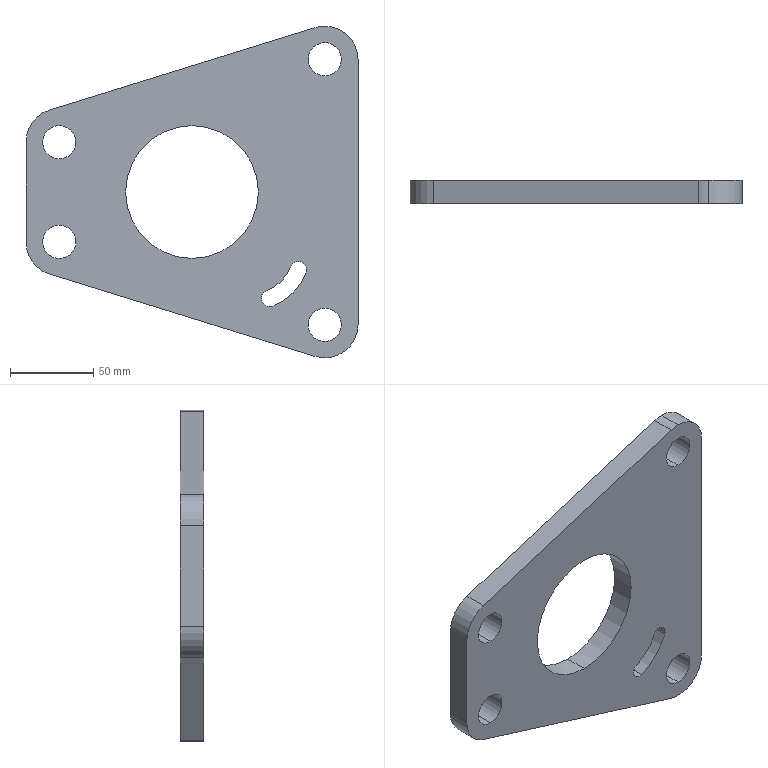Part | SolidWorks | features FlatPattern 1, SMBaseFlange 1, SheetMetal 1 | 1 solid | 26 faces | box 200 x 14 x 199.722 mm | volume 327210 mm3 | cylinder 20 | plane 6 | commonest cylinder face diameters 20 x8 40 x5 10 x3 80 x2 49 x1 69 x1
STEP:
#1=CARTESIAN_POINT('',(180.,-14.,70.));
#2=VERTEX_POINT('',#1);
#3=CARTESIAN_POINT('',(180.,-14.,90.));
#4=VERTEX_POINT('',#3);
#5=CARTESIAN_POINT('',(180.,-14.,80.));
#6=DIRECTION('',(0.,1.,0.));
#7=DIRECTION('',(0.,0.,-1.));
#8=AXIS2_PLACEMENT_3D('',#5,#6,#7);
#9=CIRCLE('',#8,10.);
#10=EDGE_CURVE('',#2,#4,#9,.T.);
#11=ORIENTED_EDGE('',*,*,#10,.F.);
#12=CARTESIAN_POINT('',(180.,0.,70.));
#13=VERTEX_POINT('',#12);
#14=CARTESIAN_POINT('',(180.,-14.,70.));
#15=DIRECTION('',(0.,1.,0.));
#16=VECTOR('',#15,1000.);
#17=LINE('',#14,#16);
#18=EDGE_CURVE('',#2,#13,#17,.T.);
#19=ORIENTED_EDGE('',*,*,#18,.T.);
#20=CARTESIAN_POINT('',(180.,0.,90.));
#21=VERTEX_POINT('',#20);
#22=CARTESIAN_POINT('',(180.,0.,80.));
#23=DIRECTION('',(0.,1.,0.));
#24=DIRECTION('',(0.,0.,-1.));
#25=AXIS2_PLACEMENT_3D('',#22,#23,#24);
#26=CIRCLE('',#25,10.);
#27=EDGE_CURVE('',#13,#21,#26,.T.);
#28=ORIENTED_EDGE('',*,*,#27,.T.);
#29=CARTESIAN_POINT('',(180.,-14.,90.));
#30=DIRECTION('',(0.,1.,0.));
#31=VECTOR('',#30,1000.);
#32=LINE('',#29,#31);
#33=EDGE_CURVE('',#4,#21,#32,.T.);
#34=ORIENTED_EDGE('',*,*,#33,.F.);
#35=EDGE_LOOP('',(#11,#19,#28,#34));
#36=FACE_OUTER_BOUND('',#35,.T.);
#37=CARTESIAN_POINT('',(180.,-14.,80.));
#38=DIRECTION('',(0.,1.,0.));
#39=DIRECTION('',(0.,0.,1.));
#40=AXIS2_PLACEMENT_3D('',#37,#38,#39);
#41=CYLINDRICAL_SURFACE('',#40,10.);
#42=ADVANCED_FACE('',(#36),#41,.F.);
#43=CARTESIAN_POINT('',(164.,-14.,-42.));
#44=VERTEX_POINT('',#43);
#45=CARTESIAN_POINT('',(168.669,-14.,-48.788));
#46=VERTEX_POINT('',#45);
#47=CARTESIAN_POINT('',(164.,-14.,-47.));
#48=DIRECTION('',(0.,1.,0.));
#49=DIRECTION('',(0.,0.,1.));
#50=AXIS2_PLACEMENT_3D('',#47,#48,#49);
#51=CIRCLE('',#50,5.);
#52=EDGE_CURVE('',#44,#46,#51,.T.);
#53=ORIENTED_EDGE('',*,*,#52,.F.);
#54=CARTESIAN_POINT('',(164.,0.,-42.));
#55=VERTEX_POINT('',#54);
#56=CARTESIAN_POINT('',(164.,-14.,-42.));
#57=DIRECTION('',(0.,1.,0.));
#58=VECTOR('',#57,1000.);
#59=LINE('',#56,#58);
#60=EDGE_CURVE('',#44,#55,#59,.T.);
#61=ORIENTED_EDGE('',*,*,#60,.T.);
#62=CARTESIAN_POINT('',(168.669,0.,-48.788));
#63=VERTEX_POINT('',#62);
#64=CARTESIAN_POINT('',(164.,0.,-47.));
#65=DIRECTION('',(0.,1.,0.));
#66=DIRECTION('',(0.,0.,1.));
#67=AXIS2_PLACEMENT_3D('',#64,#65,#66);
#68=CIRCLE('',#67,5.);
#69=EDGE_CURVE('',#55,#63,#68,.T.);
#70=ORIENTED_EDGE('',*,*,#69,.T.);
#71=CARTESIAN_POINT('',(168.669,-14.,-48.788));
#72=DIRECTION('',(0.,1.,0.));
#73=VECTOR('',#72,1000.);
#74=LINE('',#71,#73);
#75=EDGE_CURVE('',#46,#63,#74,.T.);
#76=ORIENTED_EDGE('',*,*,#75,.F.);
#77=EDGE_LOOP('',(#53,#61,#70,#76));
#78=FACE_OUTER_BOUND('',#77,.T.);
#79=CARTESIAN_POINT('',(164.,-14.,-47.));
#80=DIRECTION('',(0.,1.,0.));
#81=DIRECTION('',(0.,0.,1.));
#82=AXIS2_PLACEMENT_3D('',#79,#80,#81);
#83=CYLINDRICAL_SURFACE('',#82,5.);
#84=ADVANCED_FACE('',(#78),#83,.F.);
#85=CARTESIAN_POINT('',(20.,-14.,20.));
#86=VERTEX_POINT('',#85);
#87=CARTESIAN_POINT('',(20.,-14.,40.));
#88=VERTEX_POINT('',#87);
#89=CARTESIAN_POINT('',(20.,-14.,30.));
#90=DIRECTION('',(0.,1.,0.));
#91=DIRECTION('',(0.,0.,-1.));
#92=AXIS2_PLACEMENT_3D('',#89,#90,#91);
#93=CIRCLE('',#92,10.);
#94=EDGE_CURVE('',#86,#88,#93,.T.);
#95=ORIENTED_EDGE('',*,*,#94,.F.);
#96=CARTESIAN_POINT('',(20.,0.,20.));
#97=VERTEX_POINT('',#96);
#98=CARTESIAN_POINT('',(20.,-14.,20.));
#99=DIRECTION('',(0.,1.,0.));
#100=VECTOR('',#99,1000.);
#101=LINE('',#98,#100);
#102=EDGE_CURVE('',#86,#97,#101,.T.);
#103=ORIENTED_EDGE('',*,*,#102,.T.);
#104=CARTESIAN_POINT('',(20.,0.,40.));
#105=VERTEX_POINT('',#104);
#106=CARTESIAN_POINT('',(20.,0.,30.));
#107=DIRECTION('',(0.,1.,0.));
#108=DIRECTION('',(0.,0.,-1.));
#109=AXIS2_PLACEMENT_3D('',#106,#107,#108);
#110=CIRCLE('',#109,10.);
#111=EDGE_CURVE('',#97,#105,#110,.T.);
#112=ORIENTED_EDGE('',*,*,#111,.T.);
#113=CARTESIAN_POINT('',(20.,-14.,40.));
#114=DIRECTION('',(0.,1.,0.));
#115=VECTOR('',#114,1000.);
#116=LINE('',#113,#115);
#117=EDGE_CURVE('',#88,#105,#116,.T.);
#118=ORIENTED_EDGE('',*,*,#117,.F.);
#119=EDGE_LOOP('',(#95,#103,#112,#118));
#120=FACE_OUTER_BOUND('',#119,.T.);
#121=CARTESIAN_POINT('',(20.,-14.,30.));
#122=DIRECTION('',(0.,1.,0.));
#123=DIRECTION('',(0.,0.,1.));
#124=AXIS2_PLACEMENT_3D('',#121,#122,#123);
#125=CYLINDRICAL_SURFACE('',#124,10.);
#126=ADVANCED_FACE('',(#120),#125,.F.);
#127=CARTESIAN_POINT('',(180.,-14.,-90.));
#128=VERTEX_POINT('',#127);
#129=CARTESIAN_POINT('',(180.,-14.,-70.));
#130=VERTEX_POINT('',#129);
#131=CARTESIAN_POINT('',(180.,-14.,-80.));
#132=DIRECTION('',(0.,1.,0.));
#133=DIRECTION('',(0.,0.,1.));
#134=AXIS2_PLACEMENT_3D('',#131,#132,#133);
#135=CIRCLE('',#134,10.);
#136=EDGE_CURVE('',#128,#130,#135,.T.);
#137=ORIENTED_EDGE('',*,*,#136,.F.);
#138=CARTESIAN_POINT('',(180.,0.,-90.));
#139=VERTEX_POINT('',#138);
#140=CARTESIAN_POINT('',(180.,-14.,-90.));
#141=DIRECTION('',(0.,1.,0.));
#142=VECTOR('',#141,1000.);
#143=LINE('',#140,#142);
#144=EDGE_CURVE('',#128,#139,#143,.T.);
#145=ORIENTED_EDGE('',*,*,#144,.T.);
#146=CARTESIAN_POINT('',(180.,0.,-70.));
#147=VERTEX_POINT('',#146);
#148=CARTESIAN_POINT('',(180.,0.,-80.));
#149=DIRECTION('',(0.,1.,0.));
#150=DIRECTION('',(0.,0.,1.));
#151=AXIS2_PLACEMENT_3D('',#148,#149,#150);
#152=CIRCLE('',#151,10.);
#153=EDGE_CURVE('',#139,#147,#152,.T.);
#154=ORIENTED_EDGE('',*,*,#153,.T.);
#155=CARTESIAN_POINT('',(180.,-14.,-70.));
#156=DIRECTION('',(0.,1.,0.));
#157=VECTOR('',#156,1000.);
#158=LINE('',#155,#157);
#159=EDGE_CURVE('',#130,#147,#158,.T.);
#160=ORIENTED_EDGE('',*,*,#159,.F.);
#161=EDGE_LOOP('',(#137,#145,#154,#160));
#162=FACE_OUTER_BOUND('',#161,.T.);
#163=CARTESIAN_POINT('',(180.,-14.,-80.));
#164=DIRECTION('',(0.,1.,0.));
#165=DIRECTION('',(0.,0.,1.));
#166=AXIS2_PLACEMENT_3D('',#163,#164,#165);
#167=CYLINDRICAL_SURFACE('',#166,10.);
#168=ADVANCED_FACE('',(#162),#167,.F.);
#169=CARTESIAN_POINT('',(20.,-14.,-40.));
#170=VERTEX_POINT('',#169);
#171=CARTESIAN_POINT('',(20.,-14.,-20.));
#172=VERTEX_POINT('',#171);
#173=CARTESIAN_POINT('',(20.,-14.,-30.));
#174=DIRECTION('',(0.,1.,0.));
#175=DIRECTION('',(0.,0.,1.));
#176=AXIS2_PLACEMENT_3D('',#173,#174,#175);
#177=CIRCLE('',#176,10.);
#178=EDGE_CURVE('',#170,#172,#177,.T.);
#179=ORIENTED_EDGE('',*,*,#178,.F.);
#180=CARTESIAN_POINT('',(20.,0.,-40.));
#181=VERTEX_POINT('',#180);
#182=CARTESIAN_POINT('',(20.,-14.,-40.));
#183=DIRECTION('',(0.,1.,0.));
#184=VECTOR('',#183,1000.);
#185=LINE('',#182,#184);
#186=EDGE_CURVE('',#170,#181,#185,.T.);
#187=ORIENTED_EDGE('',*,*,#186,.T.);
#188=CARTESIAN_POINT('',(20.,0.,-20.));
#189=VERTEX_POINT('',#188);
#190=CARTESIAN_POINT('',(20.,0.,-30.));
#191=DIRECTION('',(0.,1.,0.));
#192=DIRECTION('',(0.,0.,1.));
#193=AXIS2_PLACEMENT_3D('',#190,#191,#192);
#194=CIRCLE('',#193,10.);
#195=EDGE_CURVE('',#181,#189,#194,.T.);
#196=ORIENTED_EDGE('',*,*,#195,.T.);
#197=CARTESIAN_POINT('',(20.,-14.,-20.));
#198=DIRECTION('',(0.,1.,0.));
#199=VECTOR('',#198,1000.);
#200=LINE('',#197,#199);
#201=EDGE_CURVE('',#172,#189,#200,.T.);
#202=ORIENTED_EDGE('',*,*,#201,.F.);
#203=EDGE_LOOP('',(#179,#187,#196,#202));
#204=FACE_OUTER_BOUND('',#203,.T.);
#205=CARTESIAN_POINT('',(20.,-14.,-30.));
#206=DIRECTION('',(0.,1.,0.));
#207=DIRECTION('',(0.,0.,1.));
#208=AXIS2_PLACEMENT_3D('',#205,#206,#207);
#209=CYLINDRICAL_SURFACE('',#208,10.);
#210=ADVANCED_FACE('',(#204),#209,.F.);
#211=CARTESIAN_POINT('',(100.,-14.,-40.));
#212=VERTEX_POINT('',#211);
#213=CARTESIAN_POINT('',(100.,-14.,40.));
#214=VERTEX_POINT('',#213);
#215=CARTESIAN_POINT('',(100.,-14.,0.));
#216=DIRECTION('',(0.,1.,0.));
#217=DIRECTION('',(0.,0.,1.));
#218=AXIS2_PLACEMENT_3D('',#215,#216,#217);
#219=CIRCLE('',#218,40.);
#220=EDGE_CURVE('',#212,#214,#219,.T.);
#221=ORIENTED_EDGE('',*,*,#220,.F.);
#222=CARTESIAN_POINT('',(100.,0.,-40.));
#223=VERTEX_POINT('',#222);
#224=CARTESIAN_POINT('',(100.,-14.,-40.));
#225=DIRECTION('',(0.,1.,0.));
#226=VECTOR('',#225,1000.);
#227=LINE('',#224,#226);
#228=EDGE_CURVE('',#212,#223,#227,.T.);
#229=ORIENTED_EDGE('',*,*,#228,.T.);
#230=CARTESIAN_POINT('',(100.,0.,40.));
#231=VERTEX_POINT('',#230);
#232=CARTESIAN_POINT('',(100.,0.,0.));
#233=DIRECTION('',(0.,1.,0.));
#234=DIRECTION('',(0.,0.,1.));
#235=AXIS2_PLACEMENT_3D('',#232,#233,#234);
#236=CIRCLE('',#235,40.);
#237=EDGE_CURVE('',#223,#231,#236,.T.);
#238=ORIENTED_EDGE('',*,*,#237,.T.);
#239=CARTESIAN_POINT('',(100.,-14.,40.));
#240=DIRECTION('',(0.,1.,0.));
#241=VECTOR('',#240,1000.);
#242=LINE('',#239,#241);
#243=EDGE_CURVE('',#214,#231,#242,.T.);
#244=ORIENTED_EDGE('',*,*,#243,.F.);
#245=EDGE_LOOP('',(#221,#229,#238,#244));
#246=FACE_OUTER_BOUND('',#245,.T.);
#247=CARTESIAN_POINT('',(100.,-14.,0.));
#248=DIRECTION('',(0.,1.,0.));
#249=DIRECTION('',(0.,0.,1.));
#250=AXIS2_PLACEMENT_3D('',#247,#248,#249);
#251=CYLINDRICAL_SURFACE('',#250,40.);
#252=ADVANCED_FACE('',(#246),#251,.F.);
#253=CARTESIAN_POINT('',(174.078,-14.,98.964));
#254=VERTEX_POINT('',#253);
#255=CARTESIAN_POINT('',(180.,-14.,99.861));
#256=VERTEX_POINT('',#255);
#257=CARTESIAN_POINT('',(180.,-14.,79.861));
#258=DIRECTION('',(0.,1.,0.));
#259=DIRECTION('',(0.,0.,1.));
#260=AXIS2_PLACEMENT_3D('',#257,#258,#259);
#261=CIRCLE('',#260,20.);
#262=EDGE_CURVE('',#254,#256,#261,.T.);
#263=ORIENTED_EDGE('',*,*,#262,.T.);
#264=CARTESIAN_POINT('',(180.,0.,99.861));
#265=VERTEX_POINT('',#264);
#266=CARTESIAN_POINT('',(180.,-14.,99.861));
#267=DIRECTION('',(0.,1.,0.));
#268=VECTOR('',#267,1000.);
#269=LINE('',#266,#268);
#270=EDGE_CURVE('',#256,#265,#269,.T.);
#271=ORIENTED_EDGE('',*,*,#270,.T.);
#272=CARTESIAN_POINT('',(174.078,0.,98.964));
#273=VERTEX_POINT('',#272);
#274=CARTESIAN_POINT('',(180.,0.,79.861));
#275=DIRECTION('',(0.,1.,0.));
#276=DIRECTION('',(0.,0.,1.));
#277=AXIS2_PLACEMENT_3D('',#274,#275,#276);
#278=CIRCLE('',#277,20.);
#279=EDGE_CURVE('',#273,#265,#278,.T.);
#280=ORIENTED_EDGE('',*,*,#279,.F.);
#281=CARTESIAN_POINT('',(174.078,-14.,98.964));
#282=DIRECTION('',(0.,1.,0.));
#283=VECTOR('',#282,1000.);
#284=LINE('',#281,#283);
#285=EDGE_CURVE('',#254,#273,#284,.T.);
#286=ORIENTED_EDGE('',*,*,#285,.F.);
#287=EDGE_LOOP('',(#263,#271,#280,#286));
#288=FACE_OUTER_BOUND('',#287,.T.);
#289=CARTESIAN_POINT('',(180.,-14.,79.861));
#290=DIRECTION('',(0.,1.,0.));
#291=DIRECTION('',(0.,0.,1.));
#292=AXIS2_PLACEMENT_3D('',#289,#290,#291);
#293=CYLINDRICAL_SURFACE('',#292,20.);
#294=ADVANCED_FACE('',(#288),#293,.T.);
#295=CARTESIAN_POINT('',(200.,0.,-79.861));
#296=VERTEX_POINT('',#295);
#297=CARTESIAN_POINT('',(174.078,0.,-98.964));
#298=VERTEX_POINT('',#297);
#299=CARTESIAN_POINT('',(180.,0.,-79.861));
#300=DIRECTION('',(0.,1.,0.));
#301=DIRECTION('',(0.,0.,-1.));
#302=AXIS2_PLACEMENT_3D('',#299,#300,#301);
#303=CIRCLE('',#302,20.);
#304=EDGE_CURVE('',#296,#298,#303,.T.);
#305=ORIENTED_EDGE('',*,*,#304,.F.);
#306=CARTESIAN_POINT('',(200.,-14.,-79.861));
#307=VERTEX_POINT('',#306);
#308=CARTESIAN_POINT('',(200.,-14.,-79.861));
#309=DIRECTION('',(0.,1.,0.));
#310=VECTOR('',#309,1000.);
#311=LINE('',#308,#310);
#312=EDGE_CURVE('',#307,#296,#311,.T.);
#313=ORIENTED_EDGE('',*,*,#312,.F.);
#314=CARTESIAN_POINT('',(174.078,-14.,-98.964));
#315=VERTEX_POINT('',#314);
#316=CARTESIAN_POINT('',(180.,-14.,-79.861));
#317=DIRECTION('',(0.,1.,0.));
#318=DIRECTION('',(0.,0.,-1.));
#319=AXIS2_PLACEMENT_3D('',#316,#317,#318);
#320=CIRCLE('',#319,20.);
#321=EDGE_CURVE('',#307,#315,#320,.T.);
#322=ORIENTED_EDGE('',*,*,#321,.T.);
#323=CARTESIAN_POINT('',(174.078,-14.,-98.964));
#324=DIRECTION('',(0.,1.,0.));
#325=VECTOR('',#324,1000.);
#326=LINE('',#323,#325);
#327=EDGE_CURVE('',#315,#298,#326,.T.);
#328=ORIENTED_EDGE('',*,*,#327,.T.);
#329=EDGE_LOOP('',(#305,#313,#322,#328));
#330=FACE_OUTER_BOUND('',#329,.T.);
#331=CARTESIAN_POINT('',(180.,-14.,-79.861));
#332=DIRECTION('',(0.,1.,0.));
#333=DIRECTION('',(0.,0.,1.));
#334=AXIS2_PLACEMENT_3D('',#331,#332,#333);
#335=CYLINDRICAL_SURFACE('',#334,20.);
#336=ADVANCED_FACE('',(#330),#335,.T.);
#337=CARTESIAN_POINT('',(200.,0.,79.861));
#338=VERTEX_POINT('',#337);
#339=CARTESIAN_POINT('',(200.,0.,-79.861));
#340=DIRECTION('',(0.,0.,-1.));
#341=VECTOR('',#340,1000.);
#342=LINE('',#339,#341);
#343=EDGE_CURVE('',#338,#296,#342,.T.);
#344=ORIENTED_EDGE('',*,*,#343,.F.);
#345=CARTESIAN_POINT('',(200.,-14.,79.861));
#346=VERTEX_POINT('',#345);
#347=CARTESIAN_POINT('',(200.,-14.,79.861));
#348=DIRECTION('',(0.,1.,0.));
#349=VECTOR('',#348,1000.);
#350=LINE('',#347,#349);
#351=EDGE_CURVE('',#346,#338,#350,.T.);
#352=ORIENTED_EDGE('',*,*,#351,.F.);
#353=CARTESIAN_POINT('',(200.,-14.,-79.861));
#354=DIRECTION('',(0.,0.,-1.));
#355=VECTOR('',#354,1000.);
#356=LINE('',#353,#355);
#357=EDGE_CURVE('',#346,#307,#356,.T.);
#358=ORIENTED_EDGE('',*,*,#357,.T.);
#359=ORIENTED_EDGE('',*,*,#312,.T.);
#360=EDGE_LOOP('',(#344,#352,#358,#359));
#361=FACE_OUTER_BOUND('',#360,.T.);
#362=CARTESIAN_POINT('',(200.,-14.,-79.861));
#363=DIRECTION('',(1.,0.,0.));
#364=DIRECTION('',(0.,0.,-1.));
#365=AXIS2_PLACEMENT_3D('',#362,#363,#364);
#366=PLANE('',#365);
#367=ADVANCED_FACE('',(#361),#366,.T.);
#368=ORIENTED_EDGE('',*,*,#270,.F.);
#369=CARTESIAN_POINT('',(180.,-14.,79.861));
#370=DIRECTION('',(0.,1.,0.));
#371=DIRECTION('',(0.,0.,1.));
#372=AXIS2_PLACEMENT_3D('',#369,#370,#371);
#373=CIRCLE('',#372,20.);
#374=EDGE_CURVE('',#256,#346,#373,.T.);
#375=ORIENTED_EDGE('',*,*,#374,.T.);
#376=ORIENTED_EDGE('',*,*,#351,.T.);
#377=CARTESIAN_POINT('',(180.,0.,79.861));
#378=DIRECTION('',(0.,1.,0.));
#379=DIRECTION('',(0.,0.,1.));
#380=AXIS2_PLACEMENT_3D('',#377,#378,#379);
#381=CIRCLE('',#380,20.);
#382=EDGE_CURVE('',#265,#338,#381,.T.);
#383=ORIENTED_EDGE('',*,*,#382,.F.);
#384=EDGE_LOOP('',(#368,#375,#376,#383));
#385=FACE_OUTER_BOUND('',#384,.T.);
#386=CARTESIAN_POINT('',(180.,-14.,79.861));
#387=DIRECTION('',(0.,1.,0.));
#388=DIRECTION('',(0.,0.,1.));
#389=AXIS2_PLACEMENT_3D('',#386,#387,#388);
#390=CYLINDRICAL_SURFACE('',#389,20.);
#391=ADVANCED_FACE('',(#385),#390,.T.);
#392=CARTESIAN_POINT('',(14.078,0.,49.364));
#393=VERTEX_POINT('',#392);
#394=CARTESIAN_POINT('',(14.078,0.,49.364));
#395=DIRECTION('',(0.9552,0.,0.2961));
#396=VECTOR('',#395,1000.);
#397=LINE('',#394,#396);
#398=EDGE_CURVE('',#393,#273,#397,.T.);
#399=ORIENTED_EDGE('',*,*,#398,.F.);
#400=CARTESIAN_POINT('',(14.078,-14.,49.364));
#401=VERTEX_POINT('',#400);
#402=CARTESIAN_POINT('',(14.078,-14.,49.364));
#403=DIRECTION('',(0.,1.,0.));
#404=VECTOR('',#403,1000.);
#405=LINE('',#402,#404);
#406=EDGE_CURVE('',#401,#393,#405,.T.);
#407=ORIENTED_EDGE('',*,*,#406,.F.);
#408=CARTESIAN_POINT('',(14.078,-14.,49.364));
#409=DIRECTION('',(0.9552,0.,0.2961));
#410=VECTOR('',#409,1000.);
#411=LINE('',#408,#410);
#412=EDGE_CURVE('',#401,#254,#411,.T.);
#413=ORIENTED_EDGE('',*,*,#412,.T.);
#414=ORIENTED_EDGE('',*,*,#285,.T.);
#415=EDGE_LOOP('',(#399,#407,#413,#414));
#416=FACE_OUTER_BOUND('',#415,.T.);
#417=CARTESIAN_POINT('',(14.078,-14.,49.364));
#418=DIRECTION('',(-0.2961,0.,0.9552));
#419=DIRECTION('',(0.9552,0.,0.2961));
#420=AXIS2_PLACEMENT_3D('',#417,#418,#419);
#421=PLANE('',#420);
#422=ADVANCED_FACE('',(#416),#421,.T.);
#423=CARTESIAN_POINT('',(0.,0.,30.261));
#424=VERTEX_POINT('',#423);
#425=CARTESIAN_POINT('',(20.,0.,30.261));
#426=DIRECTION('',(0.,1.,0.));
#427=DIRECTION('',(0.,0.,1.));
#428=AXIS2_PLACEMENT_3D('',#425,#426,#427);
#429=CIRCLE('',#428,20.);
#430=EDGE_CURVE('',#424,#393,#429,.T.);
#431=ORIENTED_EDGE('',*,*,#430,.F.);
#432=CARTESIAN_POINT('',(0.,-14.,30.261));
#433=VERTEX_POINT('',#432);
#434=CARTESIAN_POINT('',(0.,-14.,30.261));
#435=DIRECTION('',(0.,1.,0.));
#436=VECTOR('',#435,1000.);
#437=LINE('',#434,#436);
#438=EDGE_CURVE('',#433,#424,#437,.T.);
#439=ORIENTED_EDGE('',*,*,#438,.F.);
#440=CARTESIAN_POINT('',(20.,-14.,30.261));
#441=DIRECTION('',(0.,1.,0.));
#442=DIRECTION('',(0.,0.,1.));
#443=AXIS2_PLACEMENT_3D('',#440,#441,#442);
#444=CIRCLE('',#443,20.);
#445=EDGE_CURVE('',#433,#401,#444,.T.);
#446=ORIENTED_EDGE('',*,*,#445,.T.);
#447=ORIENTED_EDGE('',*,*,#406,.T.);
#448=EDGE_LOOP('',(#431,#439,#446,#447));
#449=FACE_OUTER_BOUND('',#448,.T.);
#450=CARTESIAN_POINT('',(20.,-14.,30.261));
#451=DIRECTION('',(0.,1.,0.));
#452=DIRECTION('',(0.,0.,1.));
#453=AXIS2_PLACEMENT_3D('',#450,#451,#452);
#454=CYLINDRICAL_SURFACE('',#453,20.);
#455=ADVANCED_FACE('',(#449),#454,.T.);
#456=CARTESIAN_POINT('',(0.,0.,-30.261));
#457=VERTEX_POINT('',#456);
#458=CARTESIAN_POINT('',(0.,0.,30.261));
#459=DIRECTION('',(0.,0.,1.));
#460=VECTOR('',#459,1000.);
#461=LINE('',#458,#460);
#462=EDGE_CURVE('',#457,#424,#461,.T.);
#463=ORIENTED_EDGE('',*,*,#462,.F.);
#464=CARTESIAN_POINT('',(0.,-14.,-30.261));
#465=VERTEX_POINT('',#464);
#466=CARTESIAN_POINT('',(0.,-14.,-30.261));
#467=DIRECTION('',(0.,1.,0.));
#468=VECTOR('',#467,1000.);
#469=LINE('',#466,#468);
#470=EDGE_CURVE('',#465,#457,#469,.T.);
#471=ORIENTED_EDGE('',*,*,#470,.F.);
#472=CARTESIAN_POINT('',(0.,-14.,30.261));
#473=DIRECTION('',(0.,0.,1.));
#474=VECTOR('',#473,1000.);
#475=LINE('',#472,#474);
#476=EDGE_CURVE('',#465,#433,#475,.T.);
#477=ORIENTED_EDGE('',*,*,#476,.T.);
#478=ORIENTED_EDGE('',*,*,#438,.T.);
#479=EDGE_LOOP('',(#463,#471,#477,#478));
#480=FACE_OUTER_BOUND('',#479,.T.);
#481=CARTESIAN_POINT('',(0.,-14.,30.261));
#482=DIRECTION('',(-1.,0.,0.));
#483=DIRECTION('',(0.,0.,1.));
#484=AXIS2_PLACEMENT_3D('',#481,#482,#483);
#485=PLANE('',#484);
#486=ADVANCED_FACE('',(#480),#485,.T.);
#487=CARTESIAN_POINT('',(14.078,0.,-49.364));
#488=VERTEX_POINT('',#487);
#489=CARTESIAN_POINT('',(20.,0.,-30.261));
#490=DIRECTION('',(0.,1.,0.));
#491=DIRECTION('',(0.,0.,-1.));
#492=AXIS2_PLACEMENT_3D('',#489,#490,#491);
#493=CIRCLE('',#492,20.);
#494=EDGE_CURVE('',#488,#457,#493,.T.);
#495=ORIENTED_EDGE('',*,*,#494,.F.);
#496=CARTESIAN_POINT('',(14.078,-14.,-49.364));
#497=VERTEX_POINT('',#496);
#498=CARTESIAN_POINT('',(14.078,-14.,-49.364));
#499=DIRECTION('',(0.,1.,0.));
#500=VECTOR('',#499,1000.);
#501=LINE('',#498,#500);
#502=EDGE_CURVE('',#497,#488,#501,.T.);
#503=ORIENTED_EDGE('',*,*,#502,.F.);
#504=CARTESIAN_POINT('',(20.,-14.,-30.261));
#505=DIRECTION('',(0.,1.,0.));
#506=DIRECTION('',(0.,0.,-1.));
#507=AXIS2_PLACEMENT_3D('',#504,#505,#506);
#508=CIRCLE('',#507,20.);
#509=EDGE_CURVE('',#497,#465,#508,.T.);
#510=ORIENTED_EDGE('',*,*,#509,.T.);
#511=ORIENTED_EDGE('',*,*,#470,.T.);
#512=EDGE_LOOP('',(#495,#503,#510,#511));
#513=FACE_OUTER_BOUND('',#512,.T.);
#514=CARTESIAN_POINT('',(20.,-14.,-30.261));
#515=DIRECTION('',(0.,1.,0.));
#516=DIRECTION('',(0.,0.,1.));
#517=AXIS2_PLACEMENT_3D('',#514,#515,#516);
#518=CYLINDRICAL_SURFACE('',#517,20.);
#519=ADVANCED_FACE('',(#513),#518,.T.);
#520=CARTESIAN_POINT('',(14.078,0.,-49.364));
#521=DIRECTION('',(-0.9552,0.,0.2961));
#522=VECTOR('',#521,1000.);
#523=LINE('',#520,#522);
#524=EDGE_CURVE('',#298,#488,#523,.T.);
#525=ORIENTED_EDGE('',*,*,#524,.F.);
#526=ORIENTED_EDGE('',*,*,#327,.F.);
#527=CARTESIAN_POINT('',(14.078,-14.,-49.364));
#528=DIRECTION('',(-0.9552,0.,0.2961));
#529=VECTOR('',#528,1000.);
#530=LINE('',#527,#529);
#531=EDGE_CURVE('',#315,#497,#530,.T.);
#532=ORIENTED_EDGE('',*,*,#531,.T.);
#533=ORIENTED_EDGE('',*,*,#502,.T.);
#534=EDGE_LOOP('',(#525,#526,#532,#533));
#535=FACE_OUTER_BOUND('',#534,.T.);
#536=CARTESIAN_POINT('',(14.078,-14.,-49.364));
#537=DIRECTION('',(-0.2961,0.,-0.9552));
#538=DIRECTION('',(-0.9552,0.,0.2961));
#539=AXIS2_PLACEMENT_3D('',#536,#537,#538);
#540=PLANE('',#539);
#541=ADVANCED_FACE('',(#535),#540,.T.);
#542=CARTESIAN_POINT('',(180.,-14.,80.));
#543=DIRECTION('',(0.,1.,0.));
#544=DIRECTION('',(0.,0.,-1.));
#545=AXIS2_PLACEMENT_3D('',#542,#543,#544);
#546=CIRCLE('',#545,10.);
#547=EDGE_CURVE('',#4,#2,#546,.T.);
#548=ORIENTED_EDGE('',*,*,#547,.T.);
#549=ORIENTED_EDGE('',*,*,#10,.T.);
#550=EDGE_LOOP('',(#548,#549));
#551=FACE_BOUND('',#550,.T.);
#552=CARTESIAN_POINT('',(145.212,-14.,-59.331));
#553=VERTEX_POINT('',#552);
#554=CARTESIAN_POINT('',(159.331,-14.,-45.212));
#555=VERTEX_POINT('',#554);
#556=CARTESIAN_POINT('',(136.451,-14.,-36.451));
#557=DIRECTION('',(0.,-1.,0.));
#558=DIRECTION('',(0.,0.,-1.));
#559=AXIS2_PLACEMENT_3D('',#556,#557,#558);
#560=CIRCLE('',#559,24.5);
#561=EDGE_CURVE('',#553,#555,#560,.T.);
#562=ORIENTED_EDGE('',*,*,#561,.T.);
#563=CARTESIAN_POINT('',(164.,-14.,-47.));
#564=DIRECTION('',(0.,1.,0.));
#565=DIRECTION('',(0.,0.,1.));
#566=AXIS2_PLACEMENT_3D('',#563,#564,#565);
#567=CIRCLE('',#566,5.);
#568=EDGE_CURVE('',#555,#44,#567,.T.);
#569=ORIENTED_EDGE('',*,*,#568,.T.);
#570=ORIENTED_EDGE('',*,*,#52,.T.);
#571=CARTESIAN_POINT('',(148.788,-14.,-68.669));
#572=VERTEX_POINT('',#571);
#573=CARTESIAN_POINT('',(136.451,-14.,-36.451));
#574=DIRECTION('',(0.,1.,0.));
#575=DIRECTION('',(0.,0.,-1.));
#576=AXIS2_PLACEMENT_3D('',#573,#574,#575);
#577=CIRCLE('',#576,34.5);
#578=EDGE_CURVE('',#46,#572,#577,.T.);
#579=ORIENTED_EDGE('',*,*,#578,.T.);
#580=CARTESIAN_POINT('',(147.,-14.,-64.));
#581=DIRECTION('',(0.,1.,0.));
#582=DIRECTION('',(0.,0.,1.));
#583=AXIS2_PLACEMENT_3D('',#580,#581,#582);
#584=CIRCLE('',#583,5.);
#585=EDGE_CURVE('',#572,#553,#584,.T.);
#586=ORIENTED_EDGE('',*,*,#585,.T.);
#587=EDGE_LOOP('',(#562,#569,#570,#579,#586));
#588=FACE_BOUND('',#587,.T.);
#589=CARTESIAN_POINT('',(20.,-14.,30.));
#590=DIRECTION('',(0.,1.,0.));
#591=DIRECTION('',(0.,0.,-1.));
#592=AXIS2_PLACEMENT_3D('',#589,#590,#591);
#593=CIRCLE('',#592,10.);
#594=EDGE_CURVE('',#88,#86,#593,.T.);
#595=ORIENTED_EDGE('',*,*,#594,.T.);
#596=ORIENTED_EDGE('',*,*,#94,.T.);
#597=EDGE_LOOP('',(#595,#596));
#598=FACE_BOUND('',#597,.T.);
#599=CARTESIAN_POINT('',(180.,-14.,-80.));
#600=DIRECTION('',(0.,1.,0.));
#601=DIRECTION('',(0.,0.,1.));
#602=AXIS2_PLACEMENT_3D('',#599,#600,#601);
#603=CIRCLE('',#602,10.);
#604=EDGE_CURVE('',#130,#128,#603,.T.);
#605=ORIENTED_EDGE('',*,*,#604,.T.);
#606=ORIENTED_EDGE('',*,*,#136,.T.);
#607=EDGE_LOOP('',(#605,#606));
#608=FACE_BOUND('',#607,.T.);
#609=CARTESIAN_POINT('',(20.,-14.,-30.));
#610=DIRECTION('',(0.,1.,0.));
#611=DIRECTION('',(0.,0.,1.));
#612=AXIS2_PLACEMENT_3D('',#609,#610,#611);
#613=CIRCLE('',#612,10.);
#614=EDGE_CURVE('',#172,#170,#613,.T.);
#615=ORIENTED_EDGE('',*,*,#614,.T.);
#616=ORIENTED_EDGE('',*,*,#178,.T.);
#617=EDGE_LOOP('',(#615,#616));
#618=FACE_BOUND('',#617,.T.);
#619=CARTESIAN_POINT('',(100.,-14.,0.));
#620=DIRECTION('',(0.,1.,0.));
#621=DIRECTION('',(0.,0.,1.));
#622=AXIS2_PLACEMENT_3D('',#619,#620,#621);
#623=CIRCLE('',#622,40.);
#624=EDGE_CURVE('',#214,#212,#623,.T.);
#625=ORIENTED_EDGE('',*,*,#624,.T.);
#626=ORIENTED_EDGE('',*,*,#220,.T.);
#627=EDGE_LOOP('',(#625,#626));
#628=FACE_BOUND('',#627,.T.);
#629=ORIENTED_EDGE('',*,*,#321,.F.);
#630=ORIENTED_EDGE('',*,*,#357,.F.);
#631=ORIENTED_EDGE('',*,*,#374,.F.);
#632=ORIENTED_EDGE('',*,*,#262,.F.);
#633=ORIENTED_EDGE('',*,*,#412,.F.);
#634=ORIENTED_EDGE('',*,*,#445,.F.);
#635=ORIENTED_EDGE('',*,*,#476,.F.);
#636=ORIENTED_EDGE('',*,*,#509,.F.);
#637=ORIENTED_EDGE('',*,*,#531,.F.);
#638=EDGE_LOOP('',(#629,#630,#631,#632,#633,#634,#635,#636,#637));
#639=FACE_OUTER_BOUND('',#638,.T.);
#640=CARTESIAN_POINT('',(180.,-14.,-79.861));
#641=DIRECTION('',(0.,-1.,0.));
#642=DIRECTION('',(0.,0.,-1.));
#643=AXIS2_PLACEMENT_3D('',#640,#641,#642);
#644=PLANE('',#643);
#645=ADVANCED_FACE('',(#551,#588,#598,#608,#618,#628,#639),#644,.T.);
#646=CARTESIAN_POINT('',(180.,0.,80.));
#647=DIRECTION('',(0.,1.,0.));
#648=DIRECTION('',(0.,0.,-1.));
#649=AXIS2_PLACEMENT_3D('',#646,#647,#648);
#650=CIRCLE('',#649,10.);
#651=EDGE_CURVE('',#21,#13,#650,.T.);
#652=ORIENTED_EDGE('',*,*,#651,.F.);
#653=ORIENTED_EDGE('',*,*,#27,.F.);
#654=EDGE_LOOP('',(#652,#653));
#655=FACE_BOUND('',#654,.T.);
#656=CARTESIAN_POINT('',(159.331,0.,-45.212));
#657=VERTEX_POINT('',#656);
#658=CARTESIAN_POINT('',(164.,0.,-47.));
#659=DIRECTION('',(0.,1.,0.));
#660=DIRECTION('',(0.,0.,1.));
#661=AXIS2_PLACEMENT_3D('',#658,#659,#660);
#662=CIRCLE('',#661,5.);
#663=EDGE_CURVE('',#657,#55,#662,.T.);
#664=ORIENTED_EDGE('',*,*,#663,.F.);
#665=CARTESIAN_POINT('',(145.212,0.,-59.331));
#666=VERTEX_POINT('',#665);
#667=CARTESIAN_POINT('',(136.451,0.,-36.451));
#668=DIRECTION('',(0.,-1.,0.));
#669=DIRECTION('',(0.,0.,-1.));
#670=AXIS2_PLACEMENT_3D('',#667,#668,#669);
#671=CIRCLE('',#670,24.5);
#672=EDGE_CURVE('',#666,#657,#671,.T.);
#673=ORIENTED_EDGE('',*,*,#672,.F.);
#674=CARTESIAN_POINT('',(148.788,0.,-68.669));
#675=VERTEX_POINT('',#674);
#676=CARTESIAN_POINT('',(147.,0.,-64.));
#677=DIRECTION('',(0.,1.,0.));
#678=DIRECTION('',(0.,0.,1.));
#679=AXIS2_PLACEMENT_3D('',#676,#677,#678);
#680=CIRCLE('',#679,5.);
#681=EDGE_CURVE('',#675,#666,#680,.T.);
#682=ORIENTED_EDGE('',*,*,#681,.F.);
#683=CARTESIAN_POINT('',(136.451,0.,-36.451));
#684=DIRECTION('',(0.,1.,0.));
#685=DIRECTION('',(0.,0.,-1.));
#686=AXIS2_PLACEMENT_3D('',#683,#684,#685);
#687=CIRCLE('',#686,34.5);
#688=EDGE_CURVE('',#63,#675,#687,.T.);
#689=ORIENTED_EDGE('',*,*,#688,.F.);
#690=ORIENTED_EDGE('',*,*,#69,.F.);
#691=EDGE_LOOP('',(#664,#673,#682,#689,#690));
#692=FACE_BOUND('',#691,.T.);
#693=CARTESIAN_POINT('',(20.,0.,30.));
#694=DIRECTION('',(0.,1.,0.));
#695=DIRECTION('',(0.,0.,-1.));
#696=AXIS2_PLACEMENT_3D('',#693,#694,#695);
#697=CIRCLE('',#696,10.);
#698=EDGE_CURVE('',#105,#97,#697,.T.);
#699=ORIENTED_EDGE('',*,*,#698,.F.);
#700=ORIENTED_EDGE('',*,*,#111,.F.);
#701=EDGE_LOOP('',(#699,#700));
#702=FACE_BOUND('',#701,.T.);
#703=CARTESIAN_POINT('',(180.,0.,-80.));
#704=DIRECTION('',(0.,1.,0.));
#705=DIRECTION('',(0.,0.,1.));
#706=AXIS2_PLACEMENT_3D('',#703,#704,#705);
#707=CIRCLE('',#706,10.);
#708=EDGE_CURVE('',#147,#139,#707,.T.);
#709=ORIENTED_EDGE('',*,*,#708,.F.);
#710=ORIENTED_EDGE('',*,*,#153,.F.);
#711=EDGE_LOOP('',(#709,#710));
#712=FACE_BOUND('',#711,.T.);
#713=CARTESIAN_POINT('',(20.,0.,-30.));
#714=DIRECTION('',(0.,1.,0.));
#715=DIRECTION('',(0.,0.,1.));
#716=AXIS2_PLACEMENT_3D('',#713,#714,#715);
#717=CIRCLE('',#716,10.);
#718=EDGE_CURVE('',#189,#181,#717,.T.);
#719=ORIENTED_EDGE('',*,*,#718,.F.);
#720=ORIENTED_EDGE('',*,*,#195,.F.);
#721=EDGE_LOOP('',(#719,#720));
#722=FACE_BOUND('',#721,.T.);
#723=CARTESIAN_POINT('',(100.,0.,0.));
#724=DIRECTION('',(0.,1.,0.));
#725=DIRECTION('',(0.,0.,1.));
#726=AXIS2_PLACEMENT_3D('',#723,#724,#725);
#727=CIRCLE('',#726,40.);
#728=EDGE_CURVE('',#231,#223,#727,.T.);
#729=ORIENTED_EDGE('',*,*,#728,.F.);
#730=ORIENTED_EDGE('',*,*,#237,.F.);
#731=EDGE_LOOP('',(#729,#730));
#732=FACE_BOUND('',#731,.T.);
#733=ORIENTED_EDGE('',*,*,#304,.T.);
#734=ORIENTED_EDGE('',*,*,#524,.T.);
#735=ORIENTED_EDGE('',*,*,#494,.T.);
#736=ORIENTED_EDGE('',*,*,#462,.T.);
#737=ORIENTED_EDGE('',*,*,#430,.T.);
#738=ORIENTED_EDGE('',*,*,#398,.T.);
#739=ORIENTED_EDGE('',*,*,#279,.T.);
#740=ORIENTED_EDGE('',*,*,#382,.T.);
#741=ORIENTED_EDGE('',*,*,#343,.T.);
#742=EDGE_LOOP('',(#733,#734,#735,#736,#737,#738,#739,#740,#741));
#743=FACE_OUTER_BOUND('',#742,.T.);
#744=CARTESIAN_POINT('',(180.,0.,-79.861));
#745=DIRECTION('',(0.,-1.,0.));
#746=DIRECTION('',(0.,0.,-1.));
#747=AXIS2_PLACEMENT_3D('',#744,#745,#746);
#748=PLANE('',#747);
#749=ADVANCED_FACE('',(#655,#692,#702,#712,#722,#732,#743),#748,.F.);
#750=ORIENTED_EDGE('',*,*,#228,.F.);
#751=ORIENTED_EDGE('',*,*,#624,.F.);
#752=ORIENTED_EDGE('',*,*,#243,.T.);
#753=ORIENTED_EDGE('',*,*,#728,.T.);
#754=EDGE_LOOP('',(#750,#751,#752,#753));
#755=FACE_OUTER_BOUND('',#754,.T.);
#756=CARTESIAN_POINT('',(100.,-14.,0.));
#757=DIRECTION('',(0.,1.,0.));
#758=DIRECTION('',(0.,0.,1.));
#759=AXIS2_PLACEMENT_3D('',#756,#757,#758);
#760=CYLINDRICAL_SURFACE('',#759,40.);
#761=ADVANCED_FACE('',(#755),#760,.F.);
#762=ORIENTED_EDGE('',*,*,#186,.F.);
#763=ORIENTED_EDGE('',*,*,#614,.F.);
#764=ORIENTED_EDGE('',*,*,#201,.T.);
#765=ORIENTED_EDGE('',*,*,#718,.T.);
#766=EDGE_LOOP('',(#762,#763,#764,#765));
#767=FACE_OUTER_BOUND('',#766,.T.);
#768=CARTESIAN_POINT('',(20.,-14.,-30.));
#769=DIRECTION('',(0.,1.,0.));
#770=DIRECTION('',(0.,0.,1.));
#771=AXIS2_PLACEMENT_3D('',#768,#769,#770);
#772=CYLINDRICAL_SURFACE('',#771,10.);
#773=ADVANCED_FACE('',(#767),#772,.F.);
#774=ORIENTED_EDGE('',*,*,#144,.F.);
#775=ORIENTED_EDGE('',*,*,#604,.F.);
#776=ORIENTED_EDGE('',*,*,#159,.T.);
#777=ORIENTED_EDGE('',*,*,#708,.T.);
#778=EDGE_LOOP('',(#774,#775,#776,#777));
#779=FACE_OUTER_BOUND('',#778,.T.);
#780=CARTESIAN_POINT('',(180.,-14.,-80.));
#781=DIRECTION('',(0.,1.,0.));
#782=DIRECTION('',(0.,0.,1.));
#783=AXIS2_PLACEMENT_3D('',#780,#781,#782);
#784=CYLINDRICAL_SURFACE('',#783,10.);
#785=ADVANCED_FACE('',(#779),#784,.F.);
#786=ORIENTED_EDGE('',*,*,#102,.F.);
#787=ORIENTED_EDGE('',*,*,#594,.F.);
#788=ORIENTED_EDGE('',*,*,#117,.T.);
#789=ORIENTED_EDGE('',*,*,#698,.T.);
#790=EDGE_LOOP('',(#786,#787,#788,#789));
#791=FACE_OUTER_BOUND('',#790,.T.);
#792=CARTESIAN_POINT('',(20.,-14.,30.));
#793=DIRECTION('',(0.,1.,0.));
#794=DIRECTION('',(0.,0.,1.));
#795=AXIS2_PLACEMENT_3D('',#792,#793,#794);
#796=CYLINDRICAL_SURFACE('',#795,10.);
#797=ADVANCED_FACE('',(#791),#796,.F.);
#798=ORIENTED_EDGE('',*,*,#672,.T.);
#799=CARTESIAN_POINT('',(159.331,-14.,-45.212));
#800=DIRECTION('',(0.,1.,0.));
#801=VECTOR('',#800,1000.);
#802=LINE('',#799,#801);
#803=EDGE_CURVE('',#555,#657,#802,.T.);
#804=ORIENTED_EDGE('',*,*,#803,.F.);
#805=ORIENTED_EDGE('',*,*,#561,.F.);
#806=CARTESIAN_POINT('',(145.212,-14.,-59.331));
#807=DIRECTION('',(0.,1.,0.));
#808=VECTOR('',#807,1000.);
#809=LINE('',#806,#808);
#810=EDGE_CURVE('',#553,#666,#809,.T.);
#811=ORIENTED_EDGE('',*,*,#810,.T.);
#812=EDGE_LOOP('',(#798,#804,#805,#811));
#813=FACE_OUTER_BOUND('',#812,.T.);
#814=CARTESIAN_POINT('',(136.451,-14.,-36.451));
#815=DIRECTION('',(0.,1.,0.));
#816=DIRECTION('',(0.,0.,1.));
#817=AXIS2_PLACEMENT_3D('',#814,#815,#816);
#818=CYLINDRICAL_SURFACE('',#817,24.5);
#819=ADVANCED_FACE('',(#813),#818,.T.);
#820=ORIENTED_EDGE('',*,*,#681,.T.);
#821=ORIENTED_EDGE('',*,*,#810,.F.);
#822=ORIENTED_EDGE('',*,*,#585,.F.);
#823=CARTESIAN_POINT('',(148.788,-14.,-68.669));
#824=DIRECTION('',(0.,1.,0.));
#825=VECTOR('',#824,1000.);
#826=LINE('',#823,#825);
#827=EDGE_CURVE('',#572,#675,#826,.T.);
#828=ORIENTED_EDGE('',*,*,#827,.T.);
#829=EDGE_LOOP('',(#820,#821,#822,#828));
#830=FACE_OUTER_BOUND('',#829,.T.);
#831=CARTESIAN_POINT('',(147.,-14.,-64.));
#832=DIRECTION('',(0.,1.,0.));
#833=DIRECTION('',(0.,0.,1.));
#834=AXIS2_PLACEMENT_3D('',#831,#832,#833);
#835=CYLINDRICAL_SURFACE('',#834,5.);
#836=ADVANCED_FACE('',(#830),#835,.F.);
#837=ORIENTED_EDGE('',*,*,#688,.T.);
#838=ORIENTED_EDGE('',*,*,#827,.F.);
#839=ORIENTED_EDGE('',*,*,#578,.F.);
#840=ORIENTED_EDGE('',*,*,#75,.T.);
#841=EDGE_LOOP('',(#837,#838,#839,#840));
#842=FACE_OUTER_BOUND('',#841,.T.);
#843=CARTESIAN_POINT('',(136.451,-14.,-36.451));
#844=DIRECTION('',(0.,1.,0.));
#845=DIRECTION('',(0.,0.,1.));
#846=AXIS2_PLACEMENT_3D('',#843,#844,#845);
#847=CYLINDRICAL_SURFACE('',#846,34.5);
#848=ADVANCED_FACE('',(#842),#847,.F.);
#849=ORIENTED_EDGE('',*,*,#60,.F.);
#850=ORIENTED_EDGE('',*,*,#568,.F.);
#851=ORIENTED_EDGE('',*,*,#803,.T.);
#852=ORIENTED_EDGE('',*,*,#663,.T.);
#853=EDGE_LOOP('',(#849,#850,#851,#852));
#854=FACE_OUTER_BOUND('',#853,.T.);
#855=CARTESIAN_POINT('',(164.,-14.,-47.));
#856=DIRECTION('',(0.,1.,0.));
#857=DIRECTION('',(0.,0.,1.));
#858=AXIS2_PLACEMENT_3D('',#855,#856,#857);
#859=CYLINDRICAL_SURFACE('',#858,5.);
#860=ADVANCED_FACE('',(#854),#859,.F.);
#861=ORIENTED_EDGE('',*,*,#18,.F.);
#862=ORIENTED_EDGE('',*,*,#547,.F.);
#863=ORIENTED_EDGE('',*,*,#33,.T.);
#864=ORIENTED_EDGE('',*,*,#651,.T.);
#865=EDGE_LOOP('',(#861,#862,#863,#864));
#866=FACE_OUTER_BOUND('',#865,.T.);
#867=CARTESIAN_POINT('',(180.,-14.,80.));
#868=DIRECTION('',(0.,1.,0.));
#869=DIRECTION('',(0.,0.,1.));
#870=AXIS2_PLACEMENT_3D('',#867,#868,#869);
#871=CYLINDRICAL_SURFACE('',#870,10.);
#872=ADVANCED_FACE('',(#866),#871,.F.);
#873=CLOSED_SHELL('',(#42,#84,#126,#168,#210,#252,#294,#336,#367,#391,#422,#455,#486,#519,#541,#645,#749,#761,#773,#785,#797,#819,#836,#848,#860,#872));
#874=MANIFOLD_SOLID_BREP('',#873);
#875=CARTESIAN_POINT('',(0.,0.,0.));
#876=DIRECTION('',(0.,0.,1.));
#877=DIRECTION('',(1.,0.,0.));
#878=AXIS2_PLACEMENT_3D('',#875,#876,#877);
#879=(LENGTH_UNIT()NAMED_UNIT(*)SI_UNIT(.MILLI.,.METRE.));
#880=UNCERTAINTY_MEASURE_WITH_UNIT(LENGTH_MEASURE(0.00001),#879,'','');
#881=(NAMED_UNIT(*)PLANE_ANGLE_UNIT()SI_UNIT($,.RADIAN.));
#882=(NAMED_UNIT(*)SI_UNIT($,.STERADIAN.)SOLID_ANGLE_UNIT());
#883=(GEOMETRIC_REPRESENTATION_CONTEXT(3)GLOBAL_UNCERTAINTY_ASSIGNED_CONTEXT((#880))GLOBAL_UNIT_ASSIGNED_CONTEXT((#879,#881,#882))REPRESENTATION_CONTEXT('',''));
#884=ADVANCED_BREP_SHAPE_REPRESENTATION('',(#874,#878),#883);